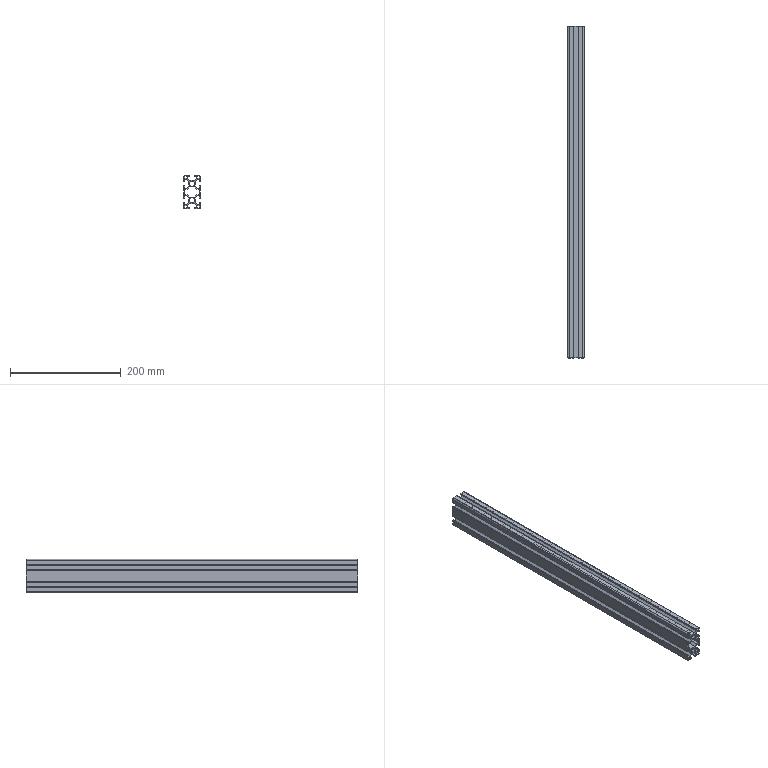Part | SolidWorks | features WeldMemberFeat 1, WeldmentFeature 1 | 1 solid | 126 faces | box 30 x 600 x 60 mm | volume 300183 mm3 | plane 118 | cylinder 8 | commonest cylinder face diameters 9.2 x4 3 x2 5 x2